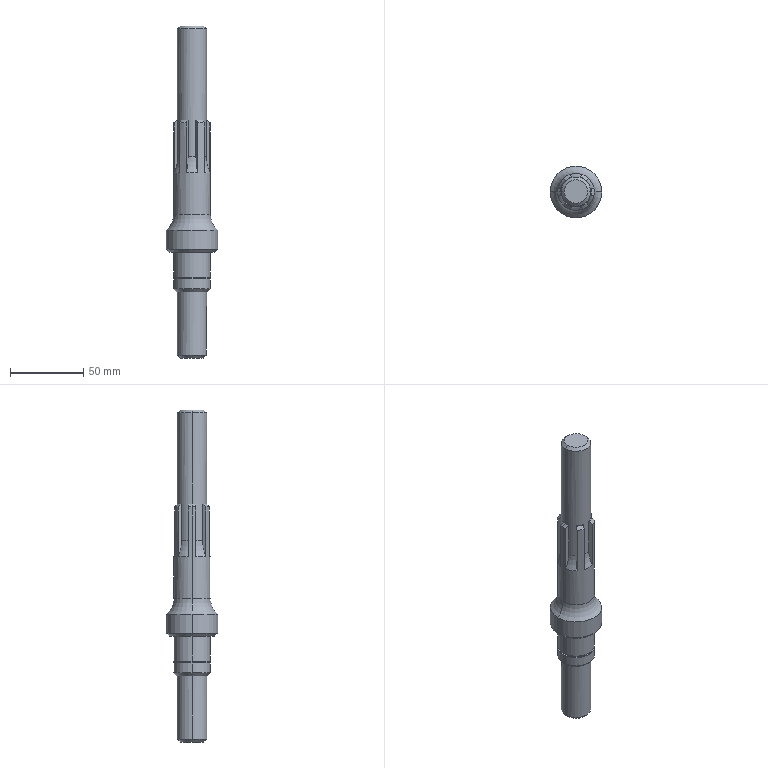Part | SolidWorks | features ICE 6, Chamfer 2, CirPattern 1, Extrusion 1, Fillet 1, RevCut 1, RevolvRefSurf 1 | 1 solid | 65 faces | box 35 x 35 x 226 mm | volume 95658 mm3 | plane 27 | cylinder 16 | cone 14 | torus 8 | commonest cylinder face diameters 25 x6 20 x4 6 x2 23 x2 35 x2